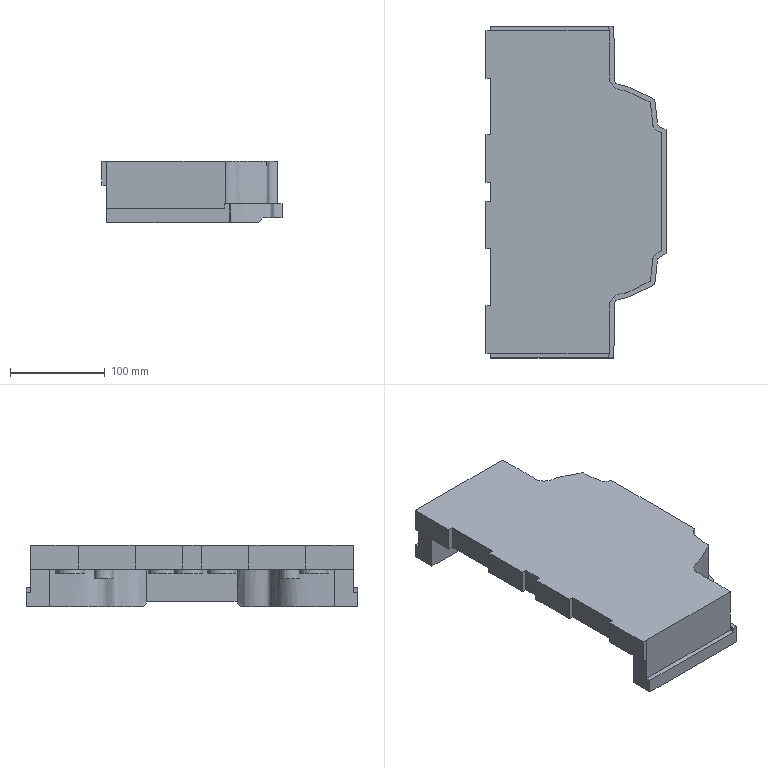Part | NX | features solid 2 | 1 solid | 62 faces | box 190 x 350.118 x 64.5 mm | volume 1931382 mm3 | plane 43 | spline 10 | cylinder 9 | commonest cylinder face diameters 30 x7 20 x2